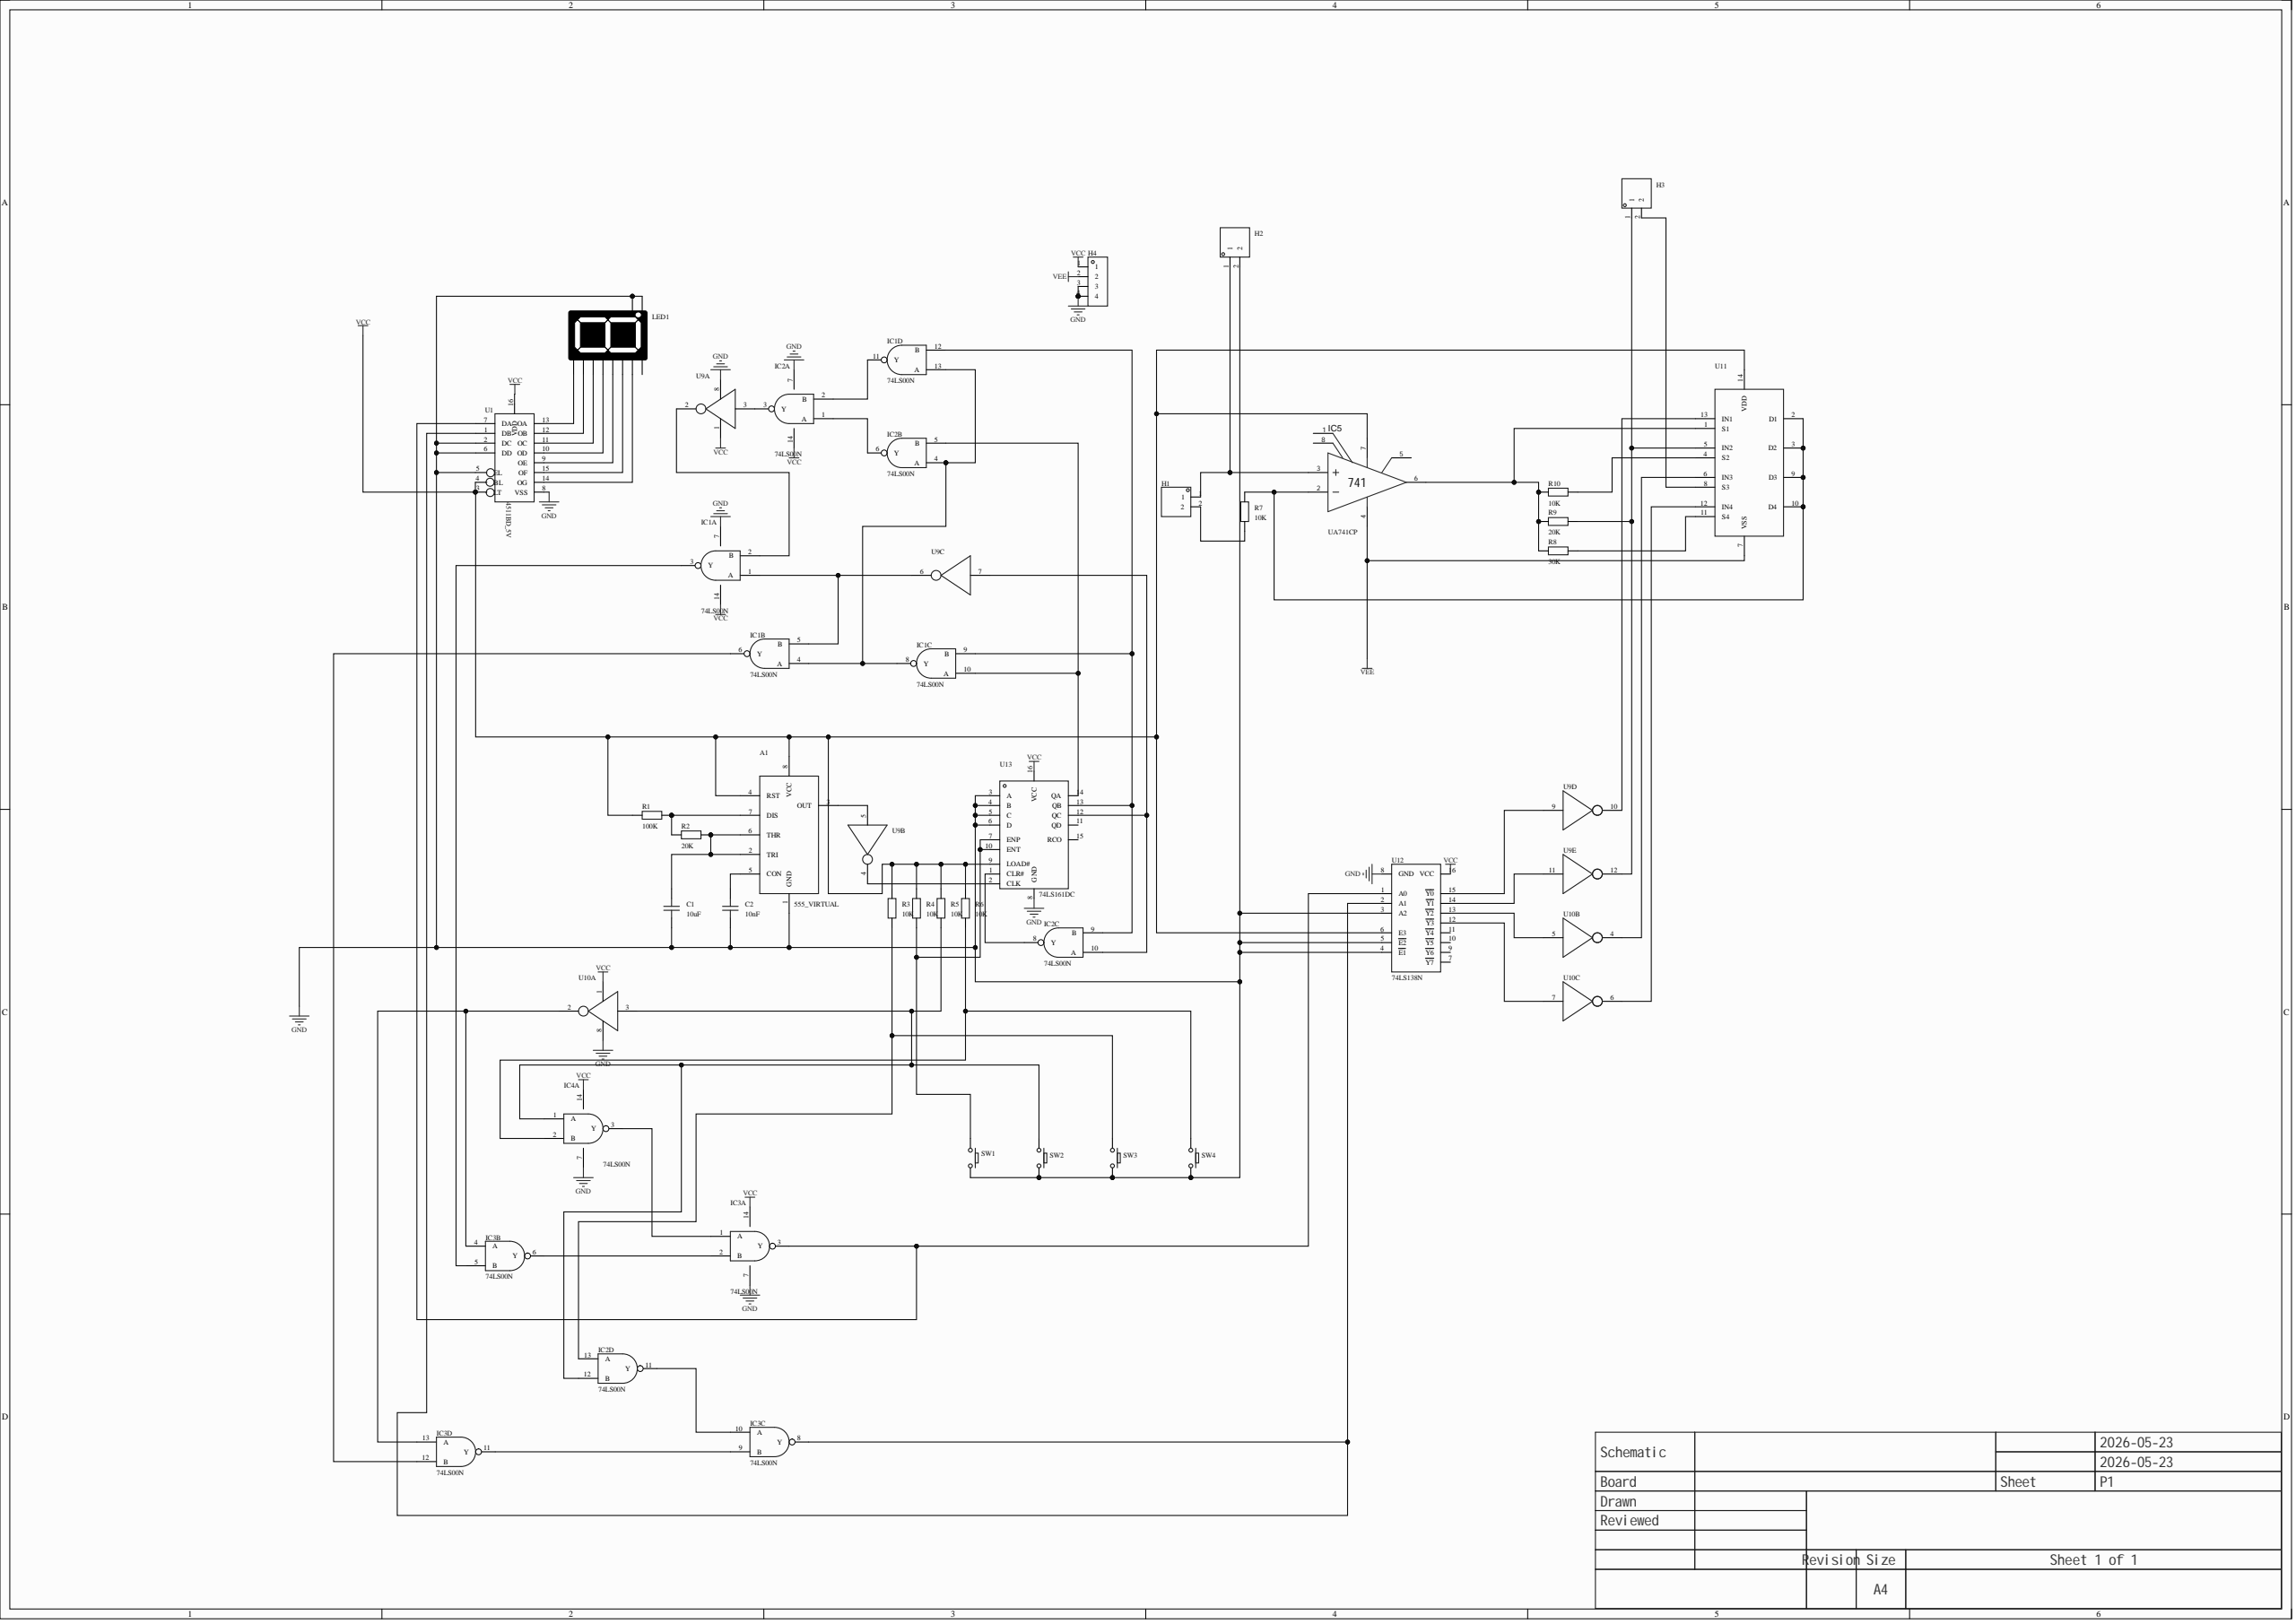Circuit board | Altium Designer | 33 parts | 54 nets
Bill of materials:
Comment,Description,Designator,Footprint,LibRef,Quantity
"555_VIRTUAL","","A1","555-VIRTUAL","555_VIRTUAL","1"
"10uF","","C1","C0805","CAP_0805","1"
"10nF","","C2","C0805","CAP_0805","1"
"","","H1, H2, H3","HDR-TH_2P-P2.54-V-M-1","HDR-M_2.54_1x2P","3"
"","","H4","HDR-TH_4P-P2.54-V-M","HDR-M_2.54_1x4P","1"
"74LS00N","","IC1, IC2, IC3, IC4","DIP14-300_MH","74LS00N","4"
"UA741CP","","IC5","DIP8","UA741CP","1"
"","","LED1","LED-SEG-TH_10P-L12.6-W19.0-P2.54-S15.24-BL","LED_SEG_TH_0.56x1","1"
"100K","","R1","R0805","Res_0805","1"
"20K","","R2, R9","R0805","Res_0805","2"
"10K","","R3, R4, R5, R6, R7, R10","R0805","Res_0805","6"
"30K","","R8","R0805","Res_0805","1"
"","","SW1, SW2, SW3, SW4","Key_TH_3.5x6x4.3","Key_TH_3.5x6x4.3","4"
"","","U1","DIP-16_L19.8-W6.5-P2.54-LS7.6-BL","4511BD_5V","1"
"","","U9, U10","PDIP-16_L19.7-W6.6-P2.54-LS7.6-BL","TC4049BP","2"
"","","U11","PDIP-14_L19.3-W6.4-P2.54-LS7.9-BL","4066BD_5V","1"
"74LS138N","","U12","DIP-16_L20.32-W6.4-P2.54-LS7.6-BL","74LS138N","1"
"74LS161DC","","U13","DIP-16_L20.32-W6.4-P2.54-LS7.6-BL","74LS161DC","1"
Netlist (Protel format):
[
A1
555-VIRTUAL
555_VIRTUAL



]
[
C1
C0805
10uF



]
[
C2
C0805
10nF



]
[
H1
HDR-TH_2P-P2.54-V-M-1




]
[
H2
HDR-TH_2P-P2.54-V-M-1




]
[
H3
HDR-TH_2P-P2.54-V-M-1




]
[
H4
HDR-TH_4P-P2.54-V-M




]
[
IC1
DIP14-300_MH
74LS00N



]
[
IC2
DIP14-300_MH
74LS00N



]
[
IC3
DIP14-300_MH
74LS00N



]
[
IC4
DIP14-300_MH
74LS00N



]
[
IC5
DIP8
UA741CP



]
[
LED1
LED-SEG-TH_10P-L12.6-W19.0-P2.54-S15.24-BL




]
[
R1
R0805
100K



]
[
R2
R0805
20K



]
[
R3
R0805
10K



]
[
R4
R0805
10K



]
[
R5
R0805
10K



]
[
R6
R0805
10K



]
[
R7
R0805
10K



]
[
R8
R0805
30K



]
[
R9
R0805
20K



]
[
R10
R0805
10K



]
[
SW1
Key_TH_3.5x6x4.3




]
[
SW2
Key_TH_3.5x6x4.3




]
[
SW3
Key_TH_3.5x6x4.3




]
[
SW4
Key_TH_3.5x6x4.3




]
[
U1
DIP-16_L19.8-W6.5-P2.54-LS7.6-BL




]
[
U9
PDIP-16_L19.7-W6.6-P2.54-LS7.6-BL




]
[
U10
PDIP-16_L19.7-W6.6-P2.54-LS7.6-BL




]
[
U11
PDIP-14_L19.3-W6.4-P2.54-LS7.9-BL




]
[
U12
DIP-16_L20.32-W6.4-P2.54-LS7.6-BL
74LS138N



]
[
U13
DIP-16_L20.32-W6.4-P2.54-LS7.6-BL
74LS161DC



]
(
VEE
H4-2
IC5-4
U11-7
)
(
VCC
H4-1
IC1-14
IC2-14
IC3-14
IC4-14
U1-3
U1-4
U1-16
U9-1
U10-1
U12-16
U13-16
)
(
NetU10_7
U10-7
U12-12
)
(
NetU10_6
U10-6
U11-12
)
(
NetU10_5
U10-5
U12-13
)
(
NetU10_4
U10-4
U11-6
)
(
NetU9_11
U9-11
U12-14
)
(
NetU9_10
U9-10
U11-13
)
(
NetU9_9
U9-9
U12-15
)
(
NetU9_4
U9-4
U13-2
)
(
NetR10_2
R10-2
U11-4
)
(
NetR8_2
R8-2
U11-11
)
(
NetR4_1
R4-1
SW1-A
U13-7
U13-10
)
(
NetLED1_10
LED1-10
U1-14
)
(
NetLED1_9
LED1-9
U1-15
)
(
NetLED1_7
LED1-7
U1-13
)
(
NetLED1_6
LED1-6
U1-12
)
(
NetLED1_4
LED1-4
U1-11
)
(
NetLED1_2
LED1-2
U1-10
)
(
NetLED1_1
LED1-1
U1-9
)
(
NetIC5_6
IC5-6
R8-1
R9-1
R10-1
U11-1
)
(
NetIC5_2
IC5-2
R7-2
U11-2
U11-3
U11-9
U11-10
)
(
NetIC4_2
IC4-2
R6-1
SW4-A
)
(
NetIC3_9
IC3-9
IC3-11
)
(
NetIC3_8
IC3-8
U1-1
U12-2
)
(
NetIC3_4
IC3-4
IC3-13
U10-2
)
(
NetIC3_3
IC3-3
U1-7
U12-1
)
(
NetIC3_2
IC3-2
IC3-6
)
(
NetIC3_1
IC3-1
IC4-3
)
(
NetIC2_13
IC2-13
R3-1
SW3-A
)
(
NetIC2_12
IC2-12
IC4-1
R5-1
SW2-A
U10-3
)
(
NetIC2_11
IC2-11
IC3-10
)
(
NetIC2_10
IC2-10
U9-7
U13-12
)
(
NetIC2_8
IC2-8
U13-1
)
(
NetIC2_3
IC2-3
U9-3
)
(
NetIC2_1
IC2-1
IC2-6
)
(
NetIC1_11
IC1-11
IC2-2
)
(
NetIC1_10
IC1-10
IC2-5
U13-14
)
(
NetIC1_9
IC1-9
IC1-12
IC2-9
U13-13
)
(
NetIC1_6
IC1-6
IC3-12
)
(
NetIC1_4
IC1-4
IC1-8
IC1-13
IC2-4
)
(
NetIC1_3
IC1-3
IC3-5
)
(
NetIC1_2
IC1-2
U9-2
)
(
NetIC1_1
IC1-1
IC1-5
U9-6
)
(
NetH3_2
H3-2
U11-8
)
(
NetH3_1
H3-1
R9-2
U9-12
U11-5
)
(
NetH1_2
H1-2
R7-1
)
(
NetH1_1
H1-1
H2-1
IC5-3
)
(
NetA1_7
A1-7
R1-2
R2-1
)
(
NetA1_5
A1-5
C2-2
)
(
NetA1_4
A1-4
A1-8
IC5-7
R1-1
R3-2
R4-2
R5-2
R6-2
U11-14
U12-6
U13-9
)
(
NetA1_3
A1-3
U9-5
)
(
NetA1_2
A1-2
A1-6
C1-2
R2-2
)
(
GND
A1-1
C1-1
C2-1
H2-2
H4-3
H4-4
IC1-7
IC2-7
IC3-7
IC4-7
LED1-3
LED1-8
SW1-B
SW2-B
SW3-B
SW4-B
U1-2
U1-5
U1-6
U1-8
U9-8
U10-8
U12-3
U12-4
U12-5
U12-8
U13-3
U13-4
U13-5
U13-6
U13-8
)